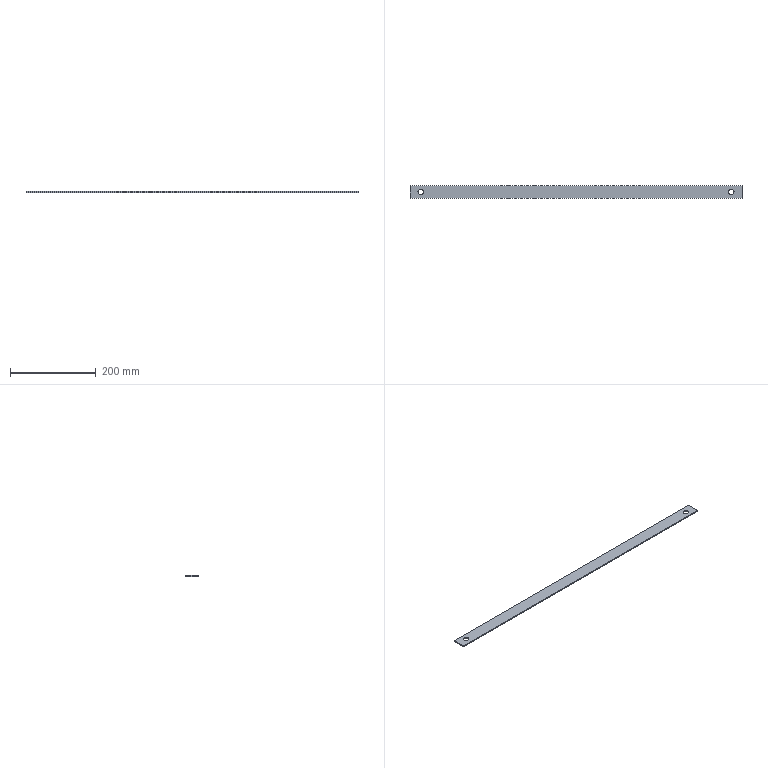Part | NX | features solid 2 | 1 solid | 10 faces | box 774 x 30 x 2.5 mm | volume 57386 mm3 | plane 6 | cylinder 4 | commonest cylinder face diameters 13 x4
STEP:
#1=CARTESIAN_POINT('',(-1088.5,277.,1295.));
#2=VERTEX_POINT('',#1);
#3=CARTESIAN_POINT('',(-1088.5,277.,1292.5));
#4=VERTEX_POINT('',#3);
#5=CARTESIAN_POINT('',(-1088.5,277.,520.415));
#6=DIRECTION('',(0.,0.,1.));
#7=VECTOR('',#6,1000.);
#8=LINE('',#5,#7);
#9=EDGE_CURVE('',#2,#4,#8,.F.);
#10=ORIENTED_EDGE('',*,*,#9,.T.);
#11=CARTESIAN_POINT('',(-1075.5,277.,1292.5));
#12=VERTEX_POINT('',#11);
#13=CARTESIAN_POINT('',(-1082.,277.,1292.5));
#14=DIRECTION('',(0.,0.,1.));
#15=DIRECTION('',(1.,0.,0.));
#16=AXIS2_PLACEMENT_3D('',#13,#14,#15);
#17=CIRCLE('',#16,6.5);
#18=EDGE_CURVE('',#12,#4,#17,.T.);
#19=ORIENTED_EDGE('',*,*,#18,.F.);
#20=CARTESIAN_POINT('',(-1075.5,277.,1295.));
#21=VERTEX_POINT('',#20);
#22=CARTESIAN_POINT('',(-1075.5,277.,520.415));
#23=DIRECTION('',(0.,0.,1.));
#24=VECTOR('',#23,1000.);
#25=LINE('',#22,#24);
#26=EDGE_CURVE('',#12,#21,#25,.T.);
#27=ORIENTED_EDGE('',*,*,#26,.T.);
#28=CARTESIAN_POINT('',(-1082.,277.,1295.));
#29=DIRECTION('',(0.,0.,1.));
#30=DIRECTION('',(1.,0.,0.));
#31=AXIS2_PLACEMENT_3D('',#28,#29,#30);
#32=CIRCLE('',#31,6.5);
#33=EDGE_CURVE('',#21,#2,#32,.T.);
#34=ORIENTED_EDGE('',*,*,#33,.T.);
#35=EDGE_LOOP('',(#10,#19,#27,#34));
#36=FACE_BOUND('',#35,.T.);
#37=CARTESIAN_POINT('',(-1082.,277.,520.415));
#38=DIRECTION('',(0.,0.,1.));
#39=DIRECTION('',(1.,0.,0.));
#40=AXIS2_PLACEMENT_3D('',#37,#38,#39);
#41=CYLINDRICAL_SURFACE('',#40,6.5);
#42=ADVANCED_FACE('',(#36),#41,.F.);
#43=CARTESIAN_POINT('',(-364.5,277.,1295.));
#44=VERTEX_POINT('',#43);
#45=CARTESIAN_POINT('',(-364.5,277.,1292.5));
#46=VERTEX_POINT('',#45);
#47=CARTESIAN_POINT('',(-364.5,277.,520.415));
#48=DIRECTION('',(0.,0.,1.));
#49=VECTOR('',#48,1000.);
#50=LINE('',#47,#49);
#51=EDGE_CURVE('',#44,#46,#50,.F.);
#52=ORIENTED_EDGE('',*,*,#51,.T.);
#53=CARTESIAN_POINT('',(-351.5,277.,1292.5));
#54=VERTEX_POINT('',#53);
#55=CARTESIAN_POINT('',(-358.,277.,1292.5));
#56=DIRECTION('',(0.,0.,1.));
#57=DIRECTION('',(1.,0.,0.));
#58=AXIS2_PLACEMENT_3D('',#55,#56,#57);
#59=CIRCLE('',#58,6.5);
#60=EDGE_CURVE('',#54,#46,#59,.T.);
#61=ORIENTED_EDGE('',*,*,#60,.F.);
#62=CARTESIAN_POINT('',(-351.5,277.,1295.));
#63=VERTEX_POINT('',#62);
#64=CARTESIAN_POINT('',(-351.5,277.,520.415));
#65=DIRECTION('',(0.,0.,1.));
#66=VECTOR('',#65,1000.);
#67=LINE('',#64,#66);
#68=EDGE_CURVE('',#54,#63,#67,.T.);
#69=ORIENTED_EDGE('',*,*,#68,.T.);
#70=CARTESIAN_POINT('',(-358.,277.,1295.));
#71=DIRECTION('',(0.,0.,1.));
#72=DIRECTION('',(1.,0.,0.));
#73=AXIS2_PLACEMENT_3D('',#70,#71,#72);
#74=CIRCLE('',#73,6.5);
#75=EDGE_CURVE('',#63,#44,#74,.T.);
#76=ORIENTED_EDGE('',*,*,#75,.T.);
#77=EDGE_LOOP('',(#52,#61,#69,#76));
#78=FACE_BOUND('',#77,.T.);
#79=CARTESIAN_POINT('',(-358.,277.,520.415));
#80=DIRECTION('',(0.,0.,1.));
#81=DIRECTION('',(1.,0.,0.));
#82=AXIS2_PLACEMENT_3D('',#79,#80,#81);
#83=CYLINDRICAL_SURFACE('',#82,6.5);
#84=ADVANCED_FACE('',(#78),#83,.F.);
#85=ORIENTED_EDGE('',*,*,#75,.F.);
#86=CARTESIAN_POINT('',(-358.,277.,1295.));
#87=DIRECTION('',(0.,0.,1.));
#88=DIRECTION('',(1.,0.,0.));
#89=AXIS2_PLACEMENT_3D('',#86,#87,#88);
#90=CIRCLE('',#89,6.5);
#91=EDGE_CURVE('',#44,#63,#90,.T.);
#92=ORIENTED_EDGE('',*,*,#91,.F.);
#93=EDGE_LOOP('',(#85,#92));
#94=FACE_BOUND('',#93,.T.);
#95=ORIENTED_EDGE('',*,*,#33,.F.);
#96=CARTESIAN_POINT('',(-1082.,277.,1295.));
#97=DIRECTION('',(0.,0.,1.));
#98=DIRECTION('',(1.,0.,0.));
#99=AXIS2_PLACEMENT_3D('',#96,#97,#98);
#100=CIRCLE('',#99,6.5);
#101=EDGE_CURVE('',#2,#21,#100,.T.);
#102=ORIENTED_EDGE('',*,*,#101,.F.);
#103=EDGE_LOOP('',(#95,#102));
#104=FACE_BOUND('',#103,.T.);
#105=CARTESIAN_POINT('',(-1107.,292.,1295.));
#106=VERTEX_POINT('',#105);
#107=CARTESIAN_POINT('',(-1107.,262.,1295.));
#108=VERTEX_POINT('',#107);
#109=CARTESIAN_POINT('',(-1107.,292.,1295.));
#110=DIRECTION('',(0.,-1.,0.));
#111=VECTOR('',#110,1000.);
#112=LINE('',#109,#111);
#113=EDGE_CURVE('',#106,#108,#112,.T.);
#114=ORIENTED_EDGE('',*,*,#113,.T.);
#115=CARTESIAN_POINT('',(-333.,262.,1295.));
#116=VERTEX_POINT('',#115);
#117=CARTESIAN_POINT('',(-1107.,262.,1295.));
#118=DIRECTION('',(1.,0.,0.));
#119=VECTOR('',#118,1000.);
#120=LINE('',#117,#119);
#121=EDGE_CURVE('',#108,#116,#120,.T.);
#122=ORIENTED_EDGE('',*,*,#121,.T.);
#123=CARTESIAN_POINT('',(-333.,292.,1295.));
#124=VERTEX_POINT('',#123);
#125=CARTESIAN_POINT('',(-333.,262.,1295.));
#126=DIRECTION('',(0.,1.,0.));
#127=VECTOR('',#126,1000.);
#128=LINE('',#125,#127);
#129=EDGE_CURVE('',#116,#124,#128,.T.);
#130=ORIENTED_EDGE('',*,*,#129,.T.);
#131=CARTESIAN_POINT('',(-333.,292.,1295.));
#132=DIRECTION('',(-1.,0.,0.));
#133=VECTOR('',#132,1000.);
#134=LINE('',#131,#133);
#135=EDGE_CURVE('',#124,#106,#134,.T.);
#136=ORIENTED_EDGE('',*,*,#135,.T.);
#137=EDGE_LOOP('',(#114,#122,#130,#136));
#138=FACE_BOUND('',#137,.T.);
#139=CARTESIAN_POINT('',(-1107.,262.,1295.));
#140=DIRECTION('',(0.,0.,1.));
#141=DIRECTION('',(0.,-1.,0.));
#142=AXIS2_PLACEMENT_3D('',#139,#140,#141);
#143=PLANE('',#142);
#144=ADVANCED_FACE('',(#94,#104,#138),#143,.T.);
#145=ORIENTED_EDGE('',*,*,#60,.T.);
#146=CARTESIAN_POINT('',(-358.,277.,1292.5));
#147=DIRECTION('',(0.,0.,1.));
#148=DIRECTION('',(1.,0.,0.));
#149=AXIS2_PLACEMENT_3D('',#146,#147,#148);
#150=CIRCLE('',#149,6.5);
#151=EDGE_CURVE('',#46,#54,#150,.T.);
#152=ORIENTED_EDGE('',*,*,#151,.T.);
#153=EDGE_LOOP('',(#145,#152));
#154=FACE_BOUND('',#153,.T.);
#155=ORIENTED_EDGE('',*,*,#18,.T.);
#156=CARTESIAN_POINT('',(-1082.,277.,1292.5));
#157=DIRECTION('',(0.,0.,1.));
#158=DIRECTION('',(1.,0.,0.));
#159=AXIS2_PLACEMENT_3D('',#156,#157,#158);
#160=CIRCLE('',#159,6.5);
#161=EDGE_CURVE('',#4,#12,#160,.T.);
#162=ORIENTED_EDGE('',*,*,#161,.T.);
#163=EDGE_LOOP('',(#155,#162));
#164=FACE_BOUND('',#163,.T.);
#165=CARTESIAN_POINT('',(-1107.,292.,1292.5));
#166=VERTEX_POINT('',#165);
#167=CARTESIAN_POINT('',(-1107.,262.,1292.5));
#168=VERTEX_POINT('',#167);
#169=CARTESIAN_POINT('',(-1107.,292.,1292.5));
#170=DIRECTION('',(0.,-1.,0.));
#171=VECTOR('',#170,1000.);
#172=LINE('',#169,#171);
#173=EDGE_CURVE('',#166,#168,#172,.T.);
#174=ORIENTED_EDGE('',*,*,#173,.F.);
#175=CARTESIAN_POINT('',(-333.,292.,1292.5));
#176=VERTEX_POINT('',#175);
#177=CARTESIAN_POINT('',(-333.,292.,1292.5));
#178=DIRECTION('',(-1.,0.,0.));
#179=VECTOR('',#178,1000.);
#180=LINE('',#177,#179);
#181=EDGE_CURVE('',#176,#166,#180,.T.);
#182=ORIENTED_EDGE('',*,*,#181,.F.);
#183=CARTESIAN_POINT('',(-333.,262.,1292.5));
#184=VERTEX_POINT('',#183);
#185=CARTESIAN_POINT('',(-333.,262.,1292.5));
#186=DIRECTION('',(0.,1.,0.));
#187=VECTOR('',#186,1000.);
#188=LINE('',#185,#187);
#189=EDGE_CURVE('',#184,#176,#188,.T.);
#190=ORIENTED_EDGE('',*,*,#189,.F.);
#191=CARTESIAN_POINT('',(-1107.,262.,1292.5));
#192=DIRECTION('',(1.,0.,0.));
#193=VECTOR('',#192,1000.);
#194=LINE('',#191,#193);
#195=EDGE_CURVE('',#168,#184,#194,.T.);
#196=ORIENTED_EDGE('',*,*,#195,.F.);
#197=EDGE_LOOP('',(#174,#182,#190,#196));
#198=FACE_BOUND('',#197,.T.);
#199=CARTESIAN_POINT('',(-1107.,262.,1292.5));
#200=DIRECTION('',(0.,0.,1.));
#201=DIRECTION('',(0.,-1.,0.));
#202=AXIS2_PLACEMENT_3D('',#199,#200,#201);
#203=PLANE('',#202);
#204=ADVANCED_FACE('',(#154,#164,#198),#203,.F.);
#205=ORIENTED_EDGE('',*,*,#135,.F.);
#206=CARTESIAN_POINT('',(-333.,292.,1292.5));
#207=DIRECTION('',(0.,0.,1.));
#208=VECTOR('',#207,1000.);
#209=LINE('',#206,#208);
#210=EDGE_CURVE('',#176,#124,#209,.T.);
#211=ORIENTED_EDGE('',*,*,#210,.F.);
#212=ORIENTED_EDGE('',*,*,#181,.T.);
#213=CARTESIAN_POINT('',(-1107.,292.,1292.5));
#214=DIRECTION('',(0.,0.,1.));
#215=VECTOR('',#214,1000.);
#216=LINE('',#213,#215);
#217=EDGE_CURVE('',#166,#106,#216,.T.);
#218=ORIENTED_EDGE('',*,*,#217,.T.);
#219=EDGE_LOOP('',(#205,#211,#212,#218));
#220=FACE_BOUND('',#219,.T.);
#221=CARTESIAN_POINT('',(-333.,292.,1292.5));
#222=DIRECTION('',(0.,1.,0.));
#223=DIRECTION('',(0.,0.,-1.));
#224=AXIS2_PLACEMENT_3D('',#221,#222,#223);
#225=PLANE('',#224);
#226=ADVANCED_FACE('',(#220),#225,.T.);
#227=ORIENTED_EDGE('',*,*,#129,.F.);
#228=CARTESIAN_POINT('',(-333.,262.,1292.5));
#229=DIRECTION('',(0.,0.,1.));
#230=VECTOR('',#229,1000.);
#231=LINE('',#228,#230);
#232=EDGE_CURVE('',#184,#116,#231,.T.);
#233=ORIENTED_EDGE('',*,*,#232,.F.);
#234=ORIENTED_EDGE('',*,*,#189,.T.);
#235=ORIENTED_EDGE('',*,*,#210,.T.);
#236=EDGE_LOOP('',(#227,#233,#234,#235));
#237=FACE_BOUND('',#236,.T.);
#238=CARTESIAN_POINT('',(-333.,262.,1292.5));
#239=DIRECTION('',(1.,0.,0.));
#240=DIRECTION('',(0.,0.,1.));
#241=AXIS2_PLACEMENT_3D('',#238,#239,#240);
#242=PLANE('',#241);
#243=ADVANCED_FACE('',(#237),#242,.T.);
#244=ORIENTED_EDGE('',*,*,#121,.F.);
#245=CARTESIAN_POINT('',(-1107.,262.,1292.5));
#246=DIRECTION('',(0.,0.,1.));
#247=VECTOR('',#246,1000.);
#248=LINE('',#245,#247);
#249=EDGE_CURVE('',#168,#108,#248,.T.);
#250=ORIENTED_EDGE('',*,*,#249,.F.);
#251=ORIENTED_EDGE('',*,*,#195,.T.);
#252=ORIENTED_EDGE('',*,*,#232,.T.);
#253=EDGE_LOOP('',(#244,#250,#251,#252));
#254=FACE_BOUND('',#253,.T.);
#255=CARTESIAN_POINT('',(-1107.,262.,1292.5));
#256=DIRECTION('',(0.,-1.,0.));
#257=DIRECTION('',(0.,0.,-1.));
#258=AXIS2_PLACEMENT_3D('',#255,#256,#257);
#259=PLANE('',#258);
#260=ADVANCED_FACE('',(#254),#259,.T.);
#261=ORIENTED_EDGE('',*,*,#113,.F.);
#262=ORIENTED_EDGE('',*,*,#217,.F.);
#263=ORIENTED_EDGE('',*,*,#173,.T.);
#264=ORIENTED_EDGE('',*,*,#249,.T.);
#265=EDGE_LOOP('',(#261,#262,#263,#264));
#266=FACE_BOUND('',#265,.T.);
#267=CARTESIAN_POINT('',(-1107.,292.,1292.5));
#268=DIRECTION('',(-1.,0.,0.));
#269=DIRECTION('',(0.,0.,1.));
#270=AXIS2_PLACEMENT_3D('',#267,#268,#269);
#271=PLANE('',#270);
#272=ADVANCED_FACE('',(#266),#271,.T.);
#273=ORIENTED_EDGE('',*,*,#151,.F.);
#274=ORIENTED_EDGE('',*,*,#51,.F.);
#275=ORIENTED_EDGE('',*,*,#91,.T.);
#276=ORIENTED_EDGE('',*,*,#68,.F.);
#277=EDGE_LOOP('',(#273,#274,#275,#276));
#278=FACE_BOUND('',#277,.T.);
#279=CARTESIAN_POINT('',(-358.,277.,520.415));
#280=DIRECTION('',(0.,0.,1.));
#281=DIRECTION('',(1.,0.,0.));
#282=AXIS2_PLACEMENT_3D('',#279,#280,#281);
#283=CYLINDRICAL_SURFACE('',#282,6.5);
#284=ADVANCED_FACE('',(#278),#283,.F.);
#285=ORIENTED_EDGE('',*,*,#161,.F.);
#286=ORIENTED_EDGE('',*,*,#9,.F.);
#287=ORIENTED_EDGE('',*,*,#101,.T.);
#288=ORIENTED_EDGE('',*,*,#26,.F.);
#289=EDGE_LOOP('',(#285,#286,#287,#288));
#290=FACE_BOUND('',#289,.T.);
#291=CARTESIAN_POINT('',(-1082.,277.,520.415));
#292=DIRECTION('',(0.,0.,1.));
#293=DIRECTION('',(1.,0.,0.));
#294=AXIS2_PLACEMENT_3D('',#291,#292,#293);
#295=CYLINDRICAL_SURFACE('',#294,6.5);
#296=ADVANCED_FACE('',(#290),#295,.F.);
#297=CLOSED_SHELL('',(#42,#84,#144,#204,#226,#243,#260,#272,#284,#296));
#298=MANIFOLD_SOLID_BREP('',#297);
#299=(LENGTH_UNIT()NAMED_UNIT(*)SI_UNIT(.MILLI.,.METRE.));
#300=UNCERTAINTY_MEASURE_WITH_UNIT(LENGTH_MEASURE(0.00001),#299,'','');
#301=(NAMED_UNIT(*)PLANE_ANGLE_UNIT()SI_UNIT($,.RADIAN.));
#302=(NAMED_UNIT(*)SI_UNIT($,.STERADIAN.)SOLID_ANGLE_UNIT());
#303=(GEOMETRIC_REPRESENTATION_CONTEXT(3)GLOBAL_UNCERTAINTY_ASSIGNED_CONTEXT((#300))GLOBAL_UNIT_ASSIGNED_CONTEXT((#299,#301,#302))REPRESENTATION_CONTEXT('',''));
#304=ADVANCED_BREP_SHAPE_REPRESENTATION('',(#298),#303);